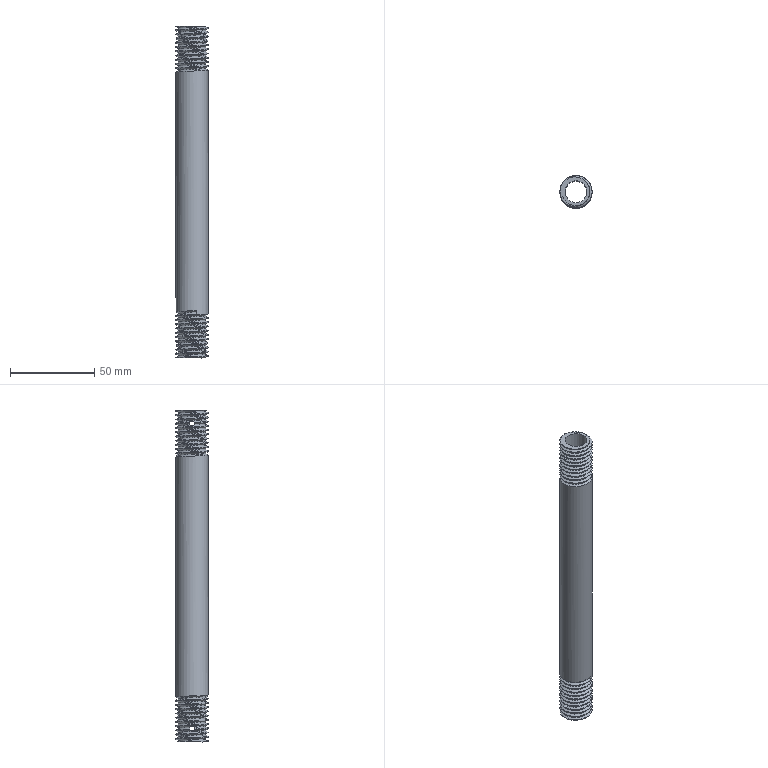Part | NX | features solid 2 | 1 solid | 44 faces | box 19.05 x 19.05 x 196.5 mm | volume 27703 mm3 | cylinder 30 | spline 10 | plane 4 | commonest cylinder face diameters 19.05 x19 16.5 x6 3 x4 13 x1